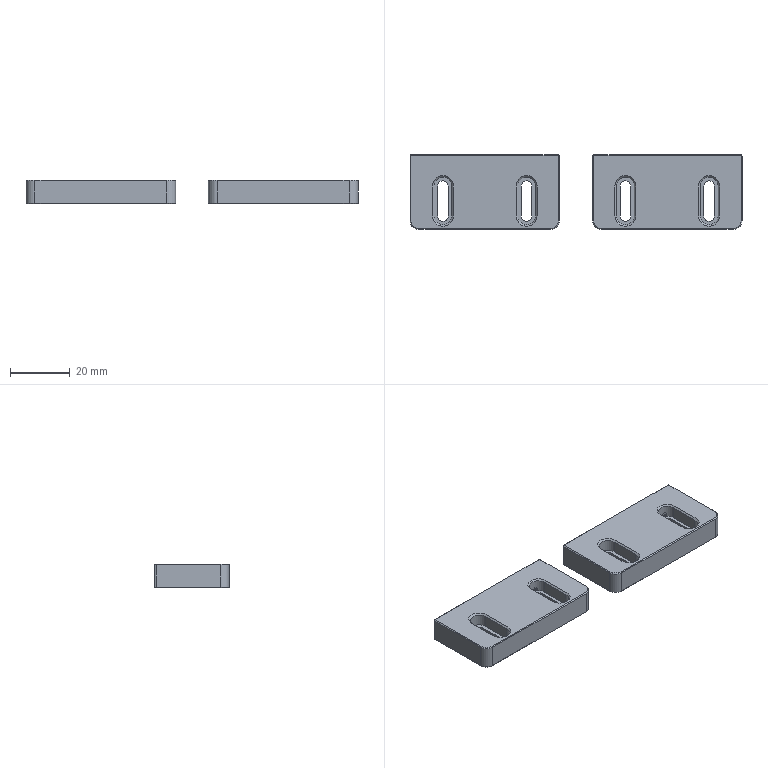NC program | NX | posted with a generic post | part box 111 x 25 x 8 mm
Whole program:
N10 G17 G21 G94 G90
(FLOOR_WALL_COPY , TOOL : D63)
N12 T01 M6
N14 G54
N16 G17 G0 G90 X90. Y0. S6500 M3
N18 G43 Z30. H1
N20 Z6.
N22 G94 G1 Z3. F1250.
N24 X87.
N26 X-87.
N28 X-90.
N30 Z6.
N32 G0 Z30.
N34 X90.
N36 Z5.
N38 G1 Z2.
N40 X87.
N42 X-87.
N44 X-90.
N46 Z5.
N48 G0 Z30.
N50 X90.
N52 Z4.
N54 G1 Z1.
N56 X87.
N58 X-87.
N60 X-90.
N62 Z4.
N64 G0 Z30.
N66 X90.
N68 Z3.
N70 G1 Z0.
N72 X87.
N74 X-87.
N76 X-90.
N78 Z3.
N80 G0 Z30.
N82 M5
(ZLEVEL_PROFILE_1_COPY_1_COPY_COPY_COPY , TOOL : D4A45)
N84 T02 M6
N86 G54
N88 G17 G0 G90 X17.291 Y-2. S9500 M3
N90 G43 Z30. H2
N92 Z1.
N94 G94 G1 Z-1. F1000.
N96 Y8.
N98 G3 X16.5 Y8.791 R0.791
N100 X15.709 Y8. R0.791
N102 G1 Y-2.
N104 G3 X16.5 Y-2.791 R0.791
N106 X17.291 Y-2. R0.791
N108 X17.091 Y-1.654 R0.4
N110 G1 Z0.
N112 G0 Z30.
N114 X43.709 Y8.
N116 Z1.
N118 G1 Z-1.
N120 Y-2.
N122 G3 X44.5 Y-2.791 R0.791
N124 X45.291 Y-2. R0.791
N126 G1 Y8.
N128 G3 X44.5 Y8.791 R0.791
N130 X43.709 Y8. R0.791
N132 X43.909 Y7.654 R0.4
N134 G1 Z0.
N136 G0 Z30.
N138 X-43.709 Y-2.
N140 Z1.
N142 G1 Z-1.
N144 Y8.
N146 G3 X-44.5 Y8.791 R0.791
N148 X-45.291 Y8. R0.791
N150 G1 Y-2.
N152 G3 X-44.5 Y-2.791 R0.791
N154 X-43.709 Y-2. R0.791
N156 X-43.909 Y-1.654 R0.4
N158 G1 Z0.
N160 G0 Z30.
N162 X-17.291 Y8.
N164 Z1.
N166 G1 Z-1.
N168 Y-2.
N170 G3 X-16.5 Y-2.791 R0.791
N172 X-15.709 Y-2. R0.791
N174 G1 Y8.
N176 G3 X-16.5 Y8.791 R0.791
N178 X-17.291 Y8. R0.791
N180 X-17.091 Y7.654 R0.4
N182 G1 Z0.
N184 G0 Z30.
N186 X-5.368 Y-13.854
N188 Z0.
N190 G1 Z-1.
N192 X-5.654 Y-13.359
N194 G3 X-6. Y-13.159 R0.4
N196 G1 X-55.
N198 G2 X-56.159 Y-12. R1.159
N200 G1 Y9.5
N202 G2 X-52.504 Y13.159 R3.659
N204 G1 X-8.5
N206 G2 X-4.841 Y9.5 R3.659
N208 G1 Y-12.
N210 G2 X-6. Y-13.159 R1.159
N212 G3 X-6.346 Y-13.359 R0.4
N214 G1 X-6.693 Y-13.959
N216 Z0.
N218 G0 Z30.
N220 X55.632 Y-13.854
N222 Z0.
N224 G1 Z-1.
N226 X55.346 Y-13.359
N228 G3 X55. Y-13.159 R0.4
N230 G1 X6.
N232 G2 X4.841 Y-12. R1.159
N234 G1 Y9.5
N236 G2 X8.504 Y13.159 R3.659
N238 G1 X52.5
N240 G2 X56.159 Y9.5 R3.659
N242 G1 Y-12.
N244 G2 X55. Y-13.159 R1.159
N246 G3 X54.654 Y-13.359 R0.4
N248 G1 X54.307 Y-13.959
N250 Z0.
N252 G0 Z30.
N254 M5
N256 M2